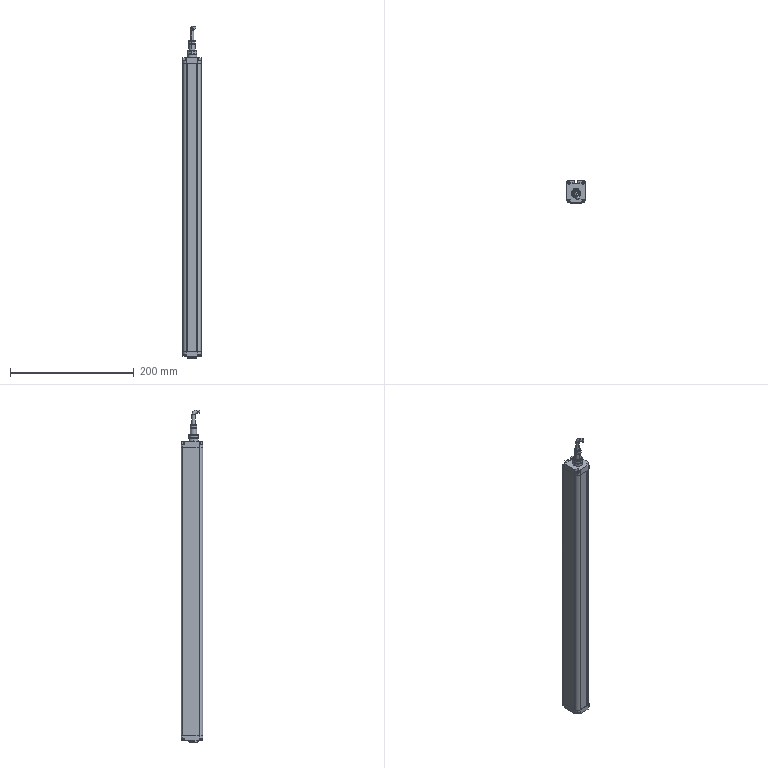Part | STEP file | Light grating 20-22 | 35 solids | 595 faces | box 30 x 35 x 536 mm | volume 422875 mm3 | plane 311 | cylinder 144 | torus 112 | cone 20 | sphere 8 | commonest cylinder face diameters 10 x46 2 x40 4 x22 1.732 x16 12 x6 5.3 x4